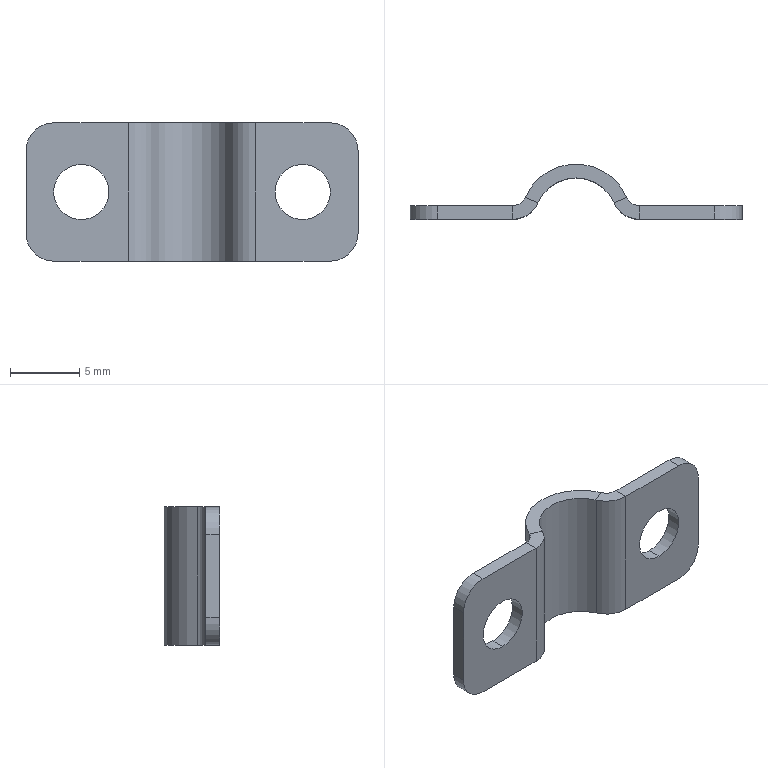Part | NX | features BREP 1 | 1 solid | 30 faces | box 24 x 4 x 10 mm | volume 235.71 mm3 | plane 16 | cylinder 14 | commonest cylinder face diameters 4 x10 2 x2 6 x1 8 x1
STEP:
#1=CARTESIAN_POINT('',(-10.,0.,5.));
#2=VERTEX_POINT('',#1);
#3=CARTESIAN_POINT('',(-12.,0.,3.));
#4=VERTEX_POINT('',#3);
#5=CARTESIAN_POINT('',(-10.,0.,3.));
#6=DIRECTION('',(0.,-1.,0.));
#7=DIRECTION('',(-1.,0.,0.));
#8=AXIS2_PLACEMENT_3D('',#5,#6,#7);
#9=CIRCLE('',#8,2.);
#10=EDGE_CURVE('',#2,#4,#9,.T.);
#11=ORIENTED_EDGE('',*,*,#10,.F.);
#12=CARTESIAN_POINT('',(-10.,1.,5.));
#13=VERTEX_POINT('',#12);
#14=CARTESIAN_POINT('',(-10.,1.6,5.));
#15=DIRECTION('',(0.,-1.,0.));
#16=VECTOR('',#15,1000.);
#17=LINE('',#14,#16);
#18=EDGE_CURVE('',#13,#2,#17,.T.);
#19=ORIENTED_EDGE('',*,*,#18,.F.);
#20=CARTESIAN_POINT('',(-12.,1.,3.));
#21=VERTEX_POINT('',#20);
#22=CARTESIAN_POINT('',(-10.,1.,3.));
#23=DIRECTION('',(0.,1.,0.));
#24=DIRECTION('',(-1.,0.,0.));
#25=AXIS2_PLACEMENT_3D('',#22,#23,#24);
#26=CIRCLE('',#25,2.);
#27=EDGE_CURVE('',#21,#13,#26,.T.);
#28=ORIENTED_EDGE('',*,*,#27,.F.);
#29=CARTESIAN_POINT('',(-12.,0.,3.));
#30=DIRECTION('',(0.,1.,0.));
#31=VECTOR('',#30,1000.);
#32=LINE('',#29,#31);
#33=EDGE_CURVE('',#4,#21,#32,.T.);
#34=ORIENTED_EDGE('',*,*,#33,.F.);
#35=EDGE_LOOP('',(#11,#19,#28,#34));
#36=FACE_BOUND('',#35,.T.);
#37=CARTESIAN_POINT('',(-10.,0.,3.));
#38=DIRECTION('',(0.,1.,0.));
#39=DIRECTION('',(0.,0.,1.));
#40=AXIS2_PLACEMENT_3D('',#37,#38,#39);
#41=CYLINDRICAL_SURFACE('',#40,2.);
#42=ADVANCED_FACE('',(#36),#41,.T.);
#43=CARTESIAN_POINT('',(-12.,0.,-3.));
#44=VERTEX_POINT('',#43);
#45=CARTESIAN_POINT('',(-10.,0.,-5.));
#46=VERTEX_POINT('',#45);
#47=CARTESIAN_POINT('',(-10.,0.,-3.));
#48=DIRECTION('',(0.,-1.,0.));
#49=DIRECTION('',(-1.,0.,0.));
#50=AXIS2_PLACEMENT_3D('',#47,#48,#49);
#51=CIRCLE('',#50,2.);
#52=EDGE_CURVE('',#44,#46,#51,.T.);
#53=ORIENTED_EDGE('',*,*,#52,.F.);
#54=CARTESIAN_POINT('',(-12.,1.,-3.));
#55=VERTEX_POINT('',#54);
#56=CARTESIAN_POINT('',(-12.,0.,-3.));
#57=DIRECTION('',(0.,-1.,0.));
#58=VECTOR('',#57,1000.);
#59=LINE('',#56,#58);
#60=EDGE_CURVE('',#55,#44,#59,.T.);
#61=ORIENTED_EDGE('',*,*,#60,.F.);
#62=CARTESIAN_POINT('',(-10.,1.,-5.));
#63=VERTEX_POINT('',#62);
#64=CARTESIAN_POINT('',(-10.,1.,-3.));
#65=DIRECTION('',(0.,1.,0.));
#66=DIRECTION('',(-1.,0.,0.));
#67=AXIS2_PLACEMENT_3D('',#64,#65,#66);
#68=CIRCLE('',#67,2.);
#69=EDGE_CURVE('',#63,#55,#68,.T.);
#70=ORIENTED_EDGE('',*,*,#69,.F.);
#71=CARTESIAN_POINT('',(-10.,1.,-5.));
#72=DIRECTION('',(0.,1.,0.));
#73=VECTOR('',#72,1000.);
#74=LINE('',#71,#73);
#75=EDGE_CURVE('',#46,#63,#74,.T.);
#76=ORIENTED_EDGE('',*,*,#75,.F.);
#77=EDGE_LOOP('',(#53,#61,#70,#76));
#78=FACE_BOUND('',#77,.T.);
#79=CARTESIAN_POINT('',(-10.,2.,-3.));
#80=DIRECTION('',(0.,-1.,0.));
#81=DIRECTION('',(0.,0.,-1.));
#82=AXIS2_PLACEMENT_3D('',#79,#80,#81);
#83=CYLINDRICAL_SURFACE('',#82,2.);
#84=ADVANCED_FACE('',(#78),#83,.T.);
#85=CARTESIAN_POINT('',(12.,1.,-3.));
#86=VERTEX_POINT('',#85);
#87=CARTESIAN_POINT('',(10.,1.,-5.));
#88=VERTEX_POINT('',#87);
#89=CARTESIAN_POINT('',(10.,1.,-3.));
#90=DIRECTION('',(0.,1.,0.));
#91=DIRECTION('',(-1.,0.,0.));
#92=AXIS2_PLACEMENT_3D('',#89,#90,#91);
#93=CIRCLE('',#92,2.);
#94=EDGE_CURVE('',#86,#88,#93,.T.);
#95=ORIENTED_EDGE('',*,*,#94,.F.);
#96=CARTESIAN_POINT('',(12.,0.,-3.));
#97=VERTEX_POINT('',#96);
#98=CARTESIAN_POINT('',(12.,1.,-3.));
#99=DIRECTION('',(0.,1.,0.));
#100=VECTOR('',#99,1000.);
#101=LINE('',#98,#100);
#102=EDGE_CURVE('',#97,#86,#101,.T.);
#103=ORIENTED_EDGE('',*,*,#102,.F.);
#104=CARTESIAN_POINT('',(10.,0.,-5.));
#105=VERTEX_POINT('',#104);
#106=CARTESIAN_POINT('',(10.,0.,-3.));
#107=DIRECTION('',(0.,-1.,0.));
#108=DIRECTION('',(-1.,0.,0.));
#109=AXIS2_PLACEMENT_3D('',#106,#107,#108);
#110=CIRCLE('',#109,2.);
#111=EDGE_CURVE('',#105,#97,#110,.T.);
#112=ORIENTED_EDGE('',*,*,#111,.F.);
#113=CARTESIAN_POINT('',(10.,1.6,-5.));
#114=DIRECTION('',(0.,-1.,0.));
#115=VECTOR('',#114,1000.);
#116=LINE('',#113,#115);
#117=EDGE_CURVE('',#88,#105,#116,.T.);
#118=ORIENTED_EDGE('',*,*,#117,.F.);
#119=EDGE_LOOP('',(#95,#103,#112,#118));
#120=FACE_BOUND('',#119,.T.);
#121=CARTESIAN_POINT('',(10.,1.6,-3.));
#122=DIRECTION('',(0.,-1.,0.));
#123=DIRECTION('',(0.,0.,-1.));
#124=AXIS2_PLACEMENT_3D('',#121,#122,#123);
#125=CYLINDRICAL_SURFACE('',#124,2.);
#126=ADVANCED_FACE('',(#120),#125,.T.);
#127=CARTESIAN_POINT('',(10.,1.,5.));
#128=VERTEX_POINT('',#127);
#129=CARTESIAN_POINT('',(12.,1.,3.));
#130=VERTEX_POINT('',#129);
#131=CARTESIAN_POINT('',(10.,1.,3.));
#132=DIRECTION('',(0.,1.,0.));
#133=DIRECTION('',(-1.,0.,0.));
#134=AXIS2_PLACEMENT_3D('',#131,#132,#133);
#135=CIRCLE('',#134,2.);
#136=EDGE_CURVE('',#128,#130,#135,.T.);
#137=ORIENTED_EDGE('',*,*,#136,.F.);
#138=CARTESIAN_POINT('',(10.,0.,5.));
#139=VERTEX_POINT('',#138);
#140=CARTESIAN_POINT('',(10.,2.,5.));
#141=DIRECTION('',(0.,1.,0.));
#142=VECTOR('',#141,1000.);
#143=LINE('',#140,#142);
#144=EDGE_CURVE('',#139,#128,#143,.T.);
#145=ORIENTED_EDGE('',*,*,#144,.F.);
#146=CARTESIAN_POINT('',(12.,0.,3.));
#147=VERTEX_POINT('',#146);
#148=CARTESIAN_POINT('',(10.,0.,3.));
#149=DIRECTION('',(0.,-1.,0.));
#150=DIRECTION('',(-1.,0.,0.));
#151=AXIS2_PLACEMENT_3D('',#148,#149,#150);
#152=CIRCLE('',#151,2.);
#153=EDGE_CURVE('',#147,#139,#152,.T.);
#154=ORIENTED_EDGE('',*,*,#153,.F.);
#155=CARTESIAN_POINT('',(12.,1.,3.));
#156=DIRECTION('',(0.,-1.,0.));
#157=VECTOR('',#156,1000.);
#158=LINE('',#155,#157);
#159=EDGE_CURVE('',#130,#147,#158,.T.);
#160=ORIENTED_EDGE('',*,*,#159,.F.);
#161=EDGE_LOOP('',(#137,#145,#154,#160));
#162=FACE_BOUND('',#161,.T.);
#163=CARTESIAN_POINT('',(10.,1.,3.));
#164=DIRECTION('',(0.,-1.,0.));
#165=DIRECTION('',(0.,0.,-1.));
#166=AXIS2_PLACEMENT_3D('',#163,#164,#165);
#167=CYLINDRICAL_SURFACE('',#166,2.);
#168=ADVANCED_FACE('',(#162),#167,.T.);
#169=CARTESIAN_POINT('',(8.,1.,-2.));
#170=VERTEX_POINT('',#169);
#171=CARTESIAN_POINT('',(8.,0.,-2.));
#172=VERTEX_POINT('',#171);
#173=CARTESIAN_POINT('',(8.,1.,-2.));
#174=DIRECTION('',(0.,1.,0.));
#175=VECTOR('',#174,1000.);
#176=LINE('',#173,#175);
#177=EDGE_CURVE('',#170,#172,#176,.F.);
#178=ORIENTED_EDGE('',*,*,#177,.T.);
#179=CARTESIAN_POINT('',(8.,0.,2.));
#180=VERTEX_POINT('',#179);
#181=CARTESIAN_POINT('',(8.,0.,0.));
#182=DIRECTION('',(0.,1.,0.));
#183=DIRECTION('',(-1.,0.,0.));
#184=AXIS2_PLACEMENT_3D('',#181,#182,#183);
#185=CIRCLE('',#184,2.);
#186=EDGE_CURVE('',#180,#172,#185,.T.);
#187=ORIENTED_EDGE('',*,*,#186,.F.);
#188=CARTESIAN_POINT('',(8.,1.,2.));
#189=VERTEX_POINT('',#188);
#190=CARTESIAN_POINT('',(8.,1.,2.));
#191=DIRECTION('',(0.,1.,0.));
#192=VECTOR('',#191,1000.);
#193=LINE('',#190,#192);
#194=EDGE_CURVE('',#189,#180,#193,.F.);
#195=ORIENTED_EDGE('',*,*,#194,.F.);
#196=CARTESIAN_POINT('',(8.,1.,0.));
#197=DIRECTION('',(0.,1.,0.));
#198=DIRECTION('',(0.,0.,1.));
#199=AXIS2_PLACEMENT_3D('',#196,#197,#198);
#200=CIRCLE('',#199,2.);
#201=EDGE_CURVE('',#189,#170,#200,.T.);
#202=ORIENTED_EDGE('',*,*,#201,.T.);
#203=EDGE_LOOP('',(#178,#187,#195,#202));
#204=FACE_BOUND('',#203,.T.);
#205=CARTESIAN_POINT('',(8.,1.,0.));
#206=DIRECTION('',(0.,1.,0.));
#207=DIRECTION('',(0.,0.,1.));
#208=AXIS2_PLACEMENT_3D('',#205,#206,#207);
#209=CYLINDRICAL_SURFACE('',#208,2.);
#210=ADVANCED_FACE('',(#204),#209,.F.);
#211=CARTESIAN_POINT('',(-8.,1.,-2.));
#212=VERTEX_POINT('',#211);
#213=CARTESIAN_POINT('',(-8.,0.,-2.));
#214=VERTEX_POINT('',#213);
#215=CARTESIAN_POINT('',(-8.,1.,-2.));
#216=DIRECTION('',(0.,1.,0.));
#217=VECTOR('',#216,1000.);
#218=LINE('',#215,#217);
#219=EDGE_CURVE('',#212,#214,#218,.F.);
#220=ORIENTED_EDGE('',*,*,#219,.T.);
#221=CARTESIAN_POINT('',(-8.,0.,2.));
#222=VERTEX_POINT('',#221);
#223=CARTESIAN_POINT('',(-8.,0.,0.));
#224=DIRECTION('',(0.,1.,0.));
#225=DIRECTION('',(-1.,0.,0.));
#226=AXIS2_PLACEMENT_3D('',#223,#224,#225);
#227=CIRCLE('',#226,2.);
#228=EDGE_CURVE('',#222,#214,#227,.T.);
#229=ORIENTED_EDGE('',*,*,#228,.F.);
#230=CARTESIAN_POINT('',(-8.,1.,2.));
#231=VERTEX_POINT('',#230);
#232=CARTESIAN_POINT('',(-8.,1.,2.));
#233=DIRECTION('',(0.,1.,0.));
#234=VECTOR('',#233,1000.);
#235=LINE('',#232,#234);
#236=EDGE_CURVE('',#231,#222,#235,.F.);
#237=ORIENTED_EDGE('',*,*,#236,.F.);
#238=CARTESIAN_POINT('',(-8.,1.,0.));
#239=DIRECTION('',(0.,1.,0.));
#240=DIRECTION('',(0.,0.,1.));
#241=AXIS2_PLACEMENT_3D('',#238,#239,#240);
#242=CIRCLE('',#241,2.);
#243=EDGE_CURVE('',#231,#212,#242,.T.);
#244=ORIENTED_EDGE('',*,*,#243,.T.);
#245=EDGE_LOOP('',(#220,#229,#237,#244));
#246=FACE_BOUND('',#245,.T.);
#247=CARTESIAN_POINT('',(-8.,1.,0.));
#248=DIRECTION('',(0.,1.,0.));
#249=DIRECTION('',(0.,0.,1.));
#250=AXIS2_PLACEMENT_3D('',#247,#248,#249);
#251=CYLINDRICAL_SURFACE('',#250,2.);
#252=ADVANCED_FACE('',(#246),#251,.F.);
#253=CARTESIAN_POINT('',(-4.583,0.,-5.));
#254=VERTEX_POINT('',#253);
#255=CARTESIAN_POINT('',(-3.,0.,-5.));
#256=DIRECTION('',(1.,0.,0.));
#257=VECTOR('',#256,1000.);
#258=LINE('',#255,#257);
#259=EDGE_CURVE('',#46,#254,#258,.T.);
#260=ORIENTED_EDGE('',*,*,#259,.F.);
#261=ORIENTED_EDGE('',*,*,#75,.T.);
#262=CARTESIAN_POINT('',(-4.583,1.,-5.));
#263=VERTEX_POINT('',#262);
#264=CARTESIAN_POINT('',(-3.,1.,-5.));
#265=DIRECTION('',(1.,0.,0.));
#266=VECTOR('',#265,1000.);
#267=LINE('',#264,#266);
#268=EDGE_CURVE('',#63,#263,#267,.T.);
#269=ORIENTED_EDGE('',*,*,#268,.T.);
#270=CARTESIAN_POINT('',(-4.583,1.,-5.));
#271=DIRECTION('',(0.,-1.,0.));
#272=VECTOR('',#271,1000.);
#273=LINE('',#270,#272);
#274=EDGE_CURVE('',#263,#254,#273,.T.);
#275=ORIENTED_EDGE('',*,*,#274,.T.);
#276=EDGE_LOOP('',(#260,#261,#269,#275));
#277=FACE_BOUND('',#276,.T.);
#278=CARTESIAN_POINT('',(4.583,2.,-5.));
#279=DIRECTION('',(0.,0.,1.));
#280=DIRECTION('',(1.,0.,0.));
#281=AXIS2_PLACEMENT_3D('',#278,#279,#280);
#282=PLANE('',#281);
#283=ADVANCED_FACE('',(#277),#282,.F.);
#284=CARTESIAN_POINT('',(4.583,0.,5.));
#285=VERTEX_POINT('',#284);
#286=CARTESIAN_POINT('',(3.,0.,5.));
#287=DIRECTION('',(1.,0.,0.));
#288=VECTOR('',#287,1000.);
#289=LINE('',#286,#288);
#290=EDGE_CURVE('',#285,#139,#289,.T.);
#291=ORIENTED_EDGE('',*,*,#290,.T.);
#292=ORIENTED_EDGE('',*,*,#144,.T.);
#293=CARTESIAN_POINT('',(4.583,1.,5.));
#294=VERTEX_POINT('',#293);
#295=CARTESIAN_POINT('',(3.,1.,5.));
#296=DIRECTION('',(1.,0.,0.));
#297=VECTOR('',#296,1000.);
#298=LINE('',#295,#297);
#299=EDGE_CURVE('',#294,#128,#298,.T.);
#300=ORIENTED_EDGE('',*,*,#299,.F.);
#301=CARTESIAN_POINT('',(4.583,1.,5.));
#302=DIRECTION('',(0.,-1.,0.));
#303=VECTOR('',#302,1000.);
#304=LINE('',#301,#303);
#305=EDGE_CURVE('',#294,#285,#304,.T.);
#306=ORIENTED_EDGE('',*,*,#305,.T.);
#307=EDGE_LOOP('',(#291,#292,#300,#306));
#308=FACE_BOUND('',#307,.T.);
#309=CARTESIAN_POINT('',(4.583,2.,5.));
#310=DIRECTION('',(0.,0.,1.));
#311=DIRECTION('',(1.,0.,0.));
#312=AXIS2_PLACEMENT_3D('',#309,#310,#311);
#313=PLANE('',#312);
#314=ADVANCED_FACE('',(#308),#313,.T.);
#315=CARTESIAN_POINT('',(2.75,1.2,-5.));
#316=VERTEX_POINT('',#315);
#317=CARTESIAN_POINT('',(4.583,0.,-5.));
#318=VERTEX_POINT('',#317);
#319=CARTESIAN_POINT('',(4.583,2.,-5.));
#320=DIRECTION('',(0.,0.,1.));
#321=DIRECTION('',(-1.,0.,0.));
#322=AXIS2_PLACEMENT_3D('',#319,#320,#321);
#323=CIRCLE('',#322,2.);
#324=EDGE_CURVE('',#316,#318,#323,.T.);
#325=ORIENTED_EDGE('',*,*,#324,.T.);
#326=CARTESIAN_POINT('',(4.583,0.,5.));
#327=DIRECTION('',(0.,0.,-1.));
#328=VECTOR('',#327,1000.);
#329=LINE('',#326,#328);
#330=EDGE_CURVE('',#285,#318,#329,.T.);
#331=ORIENTED_EDGE('',*,*,#330,.F.);
#332=CARTESIAN_POINT('',(2.75,1.2,5.));
#333=VERTEX_POINT('',#332);
#334=CARTESIAN_POINT('',(4.583,2.,5.));
#335=DIRECTION('',(0.,0.,1.));
#336=DIRECTION('',(-1.,0.,0.));
#337=AXIS2_PLACEMENT_3D('',#334,#335,#336);
#338=CIRCLE('',#337,2.);
#339=EDGE_CURVE('',#333,#285,#338,.T.);
#340=ORIENTED_EDGE('',*,*,#339,.F.);
#341=CARTESIAN_POINT('',(2.75,1.2,5.));
#342=DIRECTION('',(0.,0.,-1.));
#343=VECTOR('',#342,1000.);
#344=LINE('',#341,#343);
#345=EDGE_CURVE('',#333,#316,#344,.T.);
#346=ORIENTED_EDGE('',*,*,#345,.T.);
#347=EDGE_LOOP('',(#325,#331,#340,#346));
#348=FACE_BOUND('',#347,.T.);
#349=CARTESIAN_POINT('',(4.583,2.,5.));
#350=DIRECTION('',(0.,0.,-1.));
#351=DIRECTION('',(-1.,0.,0.));
#352=AXIS2_PLACEMENT_3D('',#349,#350,#351);
#353=CYLINDRICAL_SURFACE('',#352,2.);
#354=ADVANCED_FACE('',(#348),#353,.T.);
#355=CARTESIAN_POINT('',(-2.75,1.2,-5.));
#356=VERTEX_POINT('',#355);
#357=CARTESIAN_POINT('',(0.,0.,-5.));
#358=DIRECTION('',(0.,0.,-1.));
#359=DIRECTION('',(1.,0.,0.));
#360=AXIS2_PLACEMENT_3D('',#357,#358,#359);
#361=CIRCLE('',#360,3.);
#362=EDGE_CURVE('',#356,#316,#361,.T.);
#363=ORIENTED_EDGE('',*,*,#362,.T.);
#364=ORIENTED_EDGE('',*,*,#345,.F.);
#365=CARTESIAN_POINT('',(-2.75,1.2,5.));
#366=VERTEX_POINT('',#365);
#367=CARTESIAN_POINT('',(0.,0.,5.));
#368=DIRECTION('',(0.,0.,-1.));
#369=DIRECTION('',(1.,0.,0.));
#370=AXIS2_PLACEMENT_3D('',#367,#368,#369);
#371=CIRCLE('',#370,3.);
#372=EDGE_CURVE('',#366,#333,#371,.T.);
#373=ORIENTED_EDGE('',*,*,#372,.F.);
#374=CARTESIAN_POINT('',(-2.75,1.2,5.));
#375=DIRECTION('',(0.,0.,-1.));
#376=VECTOR('',#375,1000.);
#377=LINE('',#374,#376);
#378=EDGE_CURVE('',#366,#356,#377,.T.);
#379=ORIENTED_EDGE('',*,*,#378,.T.);
#380=EDGE_LOOP('',(#363,#364,#373,#379));
#381=FACE_BOUND('',#380,.T.);
#382=CARTESIAN_POINT('',(0.,0.,5.));
#383=DIRECTION('',(0.,0.,-1.));
#384=DIRECTION('',(-1.,0.,0.));
#385=AXIS2_PLACEMENT_3D('',#382,#383,#384);
#386=CYLINDRICAL_SURFACE('',#385,3.);
#387=ADVANCED_FACE('',(#381),#386,.F.);
#388=CARTESIAN_POINT('',(-4.583,2.,-5.));
#389=DIRECTION('',(0.,0.,1.));
#390=DIRECTION('',(-1.,0.,0.));
#391=AXIS2_PLACEMENT_3D('',#388,#389,#390);
#392=CIRCLE('',#391,2.);
#393=EDGE_CURVE('',#254,#356,#392,.T.);
#394=ORIENTED_EDGE('',*,*,#393,.T.);
#395=ORIENTED_EDGE('',*,*,#378,.F.);
#396=CARTESIAN_POINT('',(-4.583,0.,5.));
#397=VERTEX_POINT('',#396);
#398=CARTESIAN_POINT('',(-4.583,2.,5.));
#399=DIRECTION('',(0.,0.,1.));
#400=DIRECTION('',(-1.,0.,0.));
#401=AXIS2_PLACEMENT_3D('',#398,#399,#400);
#402=CIRCLE('',#401,2.);
#403=EDGE_CURVE('',#397,#366,#402,.T.);
#404=ORIENTED_EDGE('',*,*,#403,.F.);
#405=CARTESIAN_POINT('',(-4.583,0.,5.));
#406=DIRECTION('',(0.,0.,-1.));
#407=VECTOR('',#406,1000.);
#408=LINE('',#405,#407);
#409=EDGE_CURVE('',#397,#254,#408,.T.);
#410=ORIENTED_EDGE('',*,*,#409,.T.);
#411=EDGE_LOOP('',(#394,#395,#404,#410));
#412=FACE_BOUND('',#411,.T.);
#413=CARTESIAN_POINT('',(-4.583,2.,5.));
#414=DIRECTION('',(0.,0.,-1.));
#415=DIRECTION('',(-1.,0.,0.));
#416=AXIS2_PLACEMENT_3D('',#413,#414,#415);
#417=CYLINDRICAL_SURFACE('',#416,2.);
#418=ADVANCED_FACE('',(#412),#417,.T.);
#419=CARTESIAN_POINT('',(-12.,0.,5.));
#420=DIRECTION('',(0.,0.,-1.));
#421=VECTOR('',#420,1000.);
#422=LINE('',#419,#421);
#423=EDGE_CURVE('',#4,#44,#422,.T.);
#424=ORIENTED_EDGE('',*,*,#423,.T.);
#425=ORIENTED_EDGE('',*,*,#52,.T.);
#426=ORIENTED_EDGE('',*,*,#259,.T.);
#427=ORIENTED_EDGE('',*,*,#409,.F.);
#428=CARTESIAN_POINT('',(-3.,0.,5.));
#429=DIRECTION('',(1.,0.,0.));
#430=VECTOR('',#429,1000.);
#431=LINE('',#428,#430);
#432=EDGE_CURVE('',#2,#397,#431,.T.);
#433=ORIENTED_EDGE('',*,*,#432,.F.);
#434=ORIENTED_EDGE('',*,*,#10,.T.);
#435=EDGE_LOOP('',(#424,#425,#426,#427,#433,#434));
#436=FACE_BOUND('',#435,.T.);
#437=ORIENTED_EDGE('',*,*,#228,.T.);
#438=CARTESIAN_POINT('',(-8.,0.,0.));
#439=DIRECTION('',(0.,1.,0.));
#440=DIRECTION('',(-1.,0.,0.));
#441=AXIS2_PLACEMENT_3D('',#438,#439,#440);
#442=CIRCLE('',#441,2.);
#443=EDGE_CURVE('',#214,#222,#442,.T.);
#444=ORIENTED_EDGE('',*,*,#443,.T.);
#445=EDGE_LOOP('',(#437,#444));
#446=FACE_BOUND('',#445,.T.);
#447=CARTESIAN_POINT('',(-3.,0.,5.));
#448=DIRECTION('',(0.,1.,0.));
#449=DIRECTION('',(-1.,0.,0.));
#450=AXIS2_PLACEMENT_3D('',#447,#448,#449);
#451=PLANE('',#450);
#452=ADVANCED_FACE('',(#436,#446),#451,.F.);
#453=CARTESIAN_POINT('',(-12.,1.,5.));
#454=DIRECTION('',(0.,0.,-1.));
#455=VECTOR('',#454,1000.);
#456=LINE('',#453,#455);
#457=EDGE_CURVE('',#21,#55,#456,.T.);
#458=ORIENTED_EDGE('',*,*,#457,.T.);
#459=ORIENTED_EDGE('',*,*,#60,.T.);
#460=ORIENTED_EDGE('',*,*,#423,.F.);
#461=ORIENTED_EDGE('',*,*,#33,.T.);
#462=EDGE_LOOP('',(#458,#459,#460,#461));
#463=FACE_BOUND('',#462,.T.);
#464=CARTESIAN_POINT('',(-12.,0.,5.));
#465=DIRECTION('',(-1.,0.,0.));
#466=DIRECTION('',(0.,0.,1.));
#467=AXIS2_PLACEMENT_3D('',#464,#465,#466);
#468=PLANE('',#467);
#469=ADVANCED_FACE('',(#463),#468,.T.);
#470=ORIENTED_EDGE('',*,*,#268,.F.);
#471=ORIENTED_EDGE('',*,*,#69,.T.);
#472=ORIENTED_EDGE('',*,*,#457,.F.);
#473=ORIENTED_EDGE('',*,*,#27,.T.);
#474=CARTESIAN_POINT('',(-4.583,1.,5.));
#475=VERTEX_POINT('',#474);
#476=CARTESIAN_POINT('',(-3.,1.,5.));
#477=DIRECTION('',(1.,0.,0.));
#478=VECTOR('',#477,1000.);
#479=LINE('',#476,#478);
#480=EDGE_CURVE('',#13,#475,#479,.T.);
#481=ORIENTED_EDGE('',*,*,#480,.T.);
#482=CARTESIAN_POINT('',(-4.583,1.,5.));
#483=DIRECTION('',(0.,0.,-1.));
#484=VECTOR('',#483,1000.);
#485=LINE('',#482,#484);
#486=EDGE_CURVE('',#475,#263,#485,.T.);
#487=ORIENTED_EDGE('',*,*,#486,.T.);
#488=EDGE_LOOP('',(#470,#471,#472,#473,#481,#487));
#489=FACE_BOUND('',#488,.T.);
#490=ORIENTED_EDGE('',*,*,#243,.F.);
#491=CARTESIAN_POINT('',(-8.,1.,0.));
#492=DIRECTION('',(0.,1.,0.));
#493=DIRECTION('',(0.,0.,1.));
#494=AXIS2_PLACEMENT_3D('',#491,#492,#493);
#495=CIRCLE('',#494,2.);
#496=EDGE_CURVE('',#212,#231,#495,.T.);
#497=ORIENTED_EDGE('',*,*,#496,.F.);
#498=EDGE_LOOP('',(#490,#497));
#499=FACE_BOUND('',#498,.T.);
#500=CARTESIAN_POINT('',(-3.,1.,5.));
#501=DIRECTION('',(0.,1.,0.));
#502=DIRECTION('',(-1.,0.,0.));
#503=AXIS2_PLACEMENT_3D('',#500,#501,#502);
#504=PLANE('',#503);
#505=ADVANCED_FACE('',(#489,#499),#504,.T.);
#506=CARTESIAN_POINT('',(-3.666,1.6,-5.));
#507=VERTEX_POINT('',#506);
#508=CARTESIAN_POINT('',(-4.583,2.,-5.));
#509=DIRECTION('',(0.,0.,1.));
#510=DIRECTION('',(1.,0.,0.));
#511=AXIS2_PLACEMENT_3D('',#508,#509,#510);
#512=CIRCLE('',#511,1.);
#513=EDGE_CURVE('',#263,#507,#512,.T.);
#514=ORIENTED_EDGE('',*,*,#513,.F.);
#515=ORIENTED_EDGE('',*,*,#486,.F.);
#516=CARTESIAN_POINT('',(-3.666,1.6,5.));
#517=VERTEX_POINT('',#516);
#518=CARTESIAN_POINT('',(-4.583,2.,5.));
#519=DIRECTION('',(0.,0.,1.));
#520=DIRECTION('',(1.,0.,0.));
#521=AXIS2_PLACEMENT_3D('',#518,#519,#520);
#522=CIRCLE('',#521,1.);
#523=EDGE_CURVE('',#475,#517,#522,.T.);
#524=ORIENTED_EDGE('',*,*,#523,.T.);
#525=CARTESIAN_POINT('',(-3.666,1.6,5.));
#526=DIRECTION('',(0.,0.,-1.));
#527=VECTOR('',#526,1000.);
#528=LINE('',#525,#527);
#529=EDGE_CURVE('',#517,#507,#528,.T.);
#530=ORIENTED_EDGE('',*,*,#529,.T.);
#531=EDGE_LOOP('',(#514,#515,#524,#530));
#532=FACE_BOUND('',#531,.T.);
#533=CARTESIAN_POINT('',(-4.583,2.,5.));
#534=DIRECTION('',(0.,0.,-1.));
#535=DIRECTION('',(-1.,0.,0.));
#536=AXIS2_PLACEMENT_3D('',#533,#534,#535);
#537=CYLINDRICAL_SURFACE('',#536,1.);
#538=ADVANCED_FACE('',(#532),#537,.F.);
#539=CARTESIAN_POINT('',(3.666,1.6,-5.));
#540=VERTEX_POINT('',#539);
#541=CARTESIAN_POINT('',(0.,0.,-5.));
#542=DIRECTION('',(0.,0.,-1.));
#543=DIRECTION('',(1.,0.,0.));
#544=AXIS2_PLACEMENT_3D('',#541,#542,#543);
#545=CIRCLE('',#544,4.);
#546=EDGE_CURVE('',#507,#540,#545,.T.);
#547=ORIENTED_EDGE('',*,*,#546,.F.);
#548=ORIENTED_EDGE('',*,*,#529,.F.);
#549=CARTESIAN_POINT('',(3.666,1.6,5.));
#550=VERTEX_POINT('',#549);
#551=CARTESIAN_POINT('',(0.,0.,5.));
#552=DIRECTION('',(0.,0.,-1.));
#553=DIRECTION('',(1.,0.,0.));
#554=AXIS2_PLACEMENT_3D('',#551,#552,#553);
#555=CIRCLE('',#554,4.);
#556=EDGE_CURVE('',#517,#550,#555,.T.);
#557=ORIENTED_EDGE('',*,*,#556,.T.);
#558=CARTESIAN_POINT('',(3.666,1.6,5.));
#559=DIRECTION('',(0.,0.,-1.));
#560=VECTOR('',#559,1000.);
#561=LINE('',#558,#560);
#562=EDGE_CURVE('',#550,#540,#561,.T.);
#563=ORIENTED_EDGE('',*,*,#562,.T.);
#564=EDGE_LOOP('',(#547,#548,#557,#563));
#565=FACE_BOUND('',#564,.T.);
#566=CARTESIAN_POINT('',(0.,0.,5.));
#567=DIRECTION('',(0.,0.,-1.));
#568=DIRECTION('',(-1.,0.,0.));
#569=AXIS2_PLACEMENT_3D('',#566,#567,#568);
#570=CYLINDRICAL_SURFACE('',#569,4.);
#571=ADVANCED_FACE('',(#565),#570,.T.);
#572=CARTESIAN_POINT('',(4.583,1.,-5.));
#573=VERTEX_POINT('',#572);
#574=CARTESIAN_POINT('',(4.583,2.,-5.));
#575=DIRECTION('',(0.,0.,1.));
#576=DIRECTION('',(1.,0.,0.));
#577=AXIS2_PLACEMENT_3D('',#574,#575,#576);
#578=CIRCLE('',#577,1.);
#579=EDGE_CURVE('',#540,#573,#578,.T.);
#580=ORIENTED_EDGE('',*,*,#579,.F.);
#581=ORIENTED_EDGE('',*,*,#562,.F.);
#582=CARTESIAN_POINT('',(4.583,2.,5.));
#583=DIRECTION('',(0.,0.,1.));
#584=DIRECTION('',(1.,0.,0.));
#585=AXIS2_PLACEMENT_3D('',#582,#583,#584);
#586=CIRCLE('',#585,1.);
#587=EDGE_CURVE('',#550,#294,#586,.T.);
#588=ORIENTED_EDGE('',*,*,#587,.T.);
#589=CARTESIAN_POINT('',(4.583,1.,5.));
#590=DIRECTION('',(0.,0.,-1.));
#591=VECTOR('',#590,1000.);
#592=LINE('',#589,#591);
#593=EDGE_CURVE('',#294,#573,#592,.T.);
#594=ORIENTED_EDGE('',*,*,#593,.T.);
#595=EDGE_LOOP('',(#580,#581,#588,#594));
#596=FACE_BOUND('',#595,.T.);
#597=CARTESIAN_POINT('',(4.583,2.,5.));
#598=DIRECTION('',(0.,0.,-1.));
#599=DIRECTION('',(-1.,0.,0.));
#600=AXIS2_PLACEMENT_3D('',#597,#598,#599);
#601=CYLINDRICAL_SURFACE('',#600,1.);
#602=ADVANCED_FACE('',(#596),#601,.F.);
#603=ORIENTED_EDGE('',*,*,#299,.T.);
#604=ORIENTED_EDGE('',*,*,#136,.T.);
#605=CARTESIAN_POINT('',(12.,1.,5.));
#606=DIRECTION('',(0.,0.,-1.));
#607=VECTOR('',#606,1000.);
#608=LINE('',#605,#607);
#609=EDGE_CURVE('',#130,#86,#608,.T.);
#610=ORIENTED_EDGE('',*,*,#609,.T.);
#611=ORIENTED_EDGE('',*,*,#94,.T.);
#612=CARTESIAN_POINT('',(3.,1.,-5.));
#613=DIRECTION('',(1.,0.,0.));
#614=VECTOR('',#613,1000.);
#615=LINE('',#612,#614);
#616=EDGE_CURVE('',#573,#88,#615,.T.);
#617=ORIENTED_EDGE('',*,*,#616,.F.);
#618=ORIENTED_EDGE('',*,*,#593,.F.);
#619=EDGE_LOOP('',(#603,#604,#610,#611,#617,#618));
#620=FACE_BOUND('',#619,.T.);
#621=ORIENTED_EDGE('',*,*,#201,.F.);
#622=CARTESIAN_POINT('',(8.,1.,0.));
#623=DIRECTION('',(0.,1.,0.));
#624=DIRECTION('',(0.,0.,1.));
#625=AXIS2_PLACEMENT_3D('',#622,#623,#624);
#626=CIRCLE('',#625,2.);
#627=EDGE_CURVE('',#170,#189,#626,.T.);
#628=ORIENTED_EDGE('',*,*,#627,.F.);
#629=EDGE_LOOP('',(#621,#628));
#630=FACE_BOUND('',#629,.T.);
#631=CARTESIAN_POINT('',(3.,1.,5.));
#632=DIRECTION('',(0.,1.,0.));
#633=DIRECTION('',(-1.,0.,0.));
#634=AXIS2_PLACEMENT_3D('',#631,#632,#633);
#635=PLANE('',#634);
#636=ADVANCED_FACE('',(#620,#630),#635,.T.);
#637=ORIENTED_EDGE('',*,*,#609,.F.);
#638=ORIENTED_EDGE('',*,*,#159,.T.);
#639=CARTESIAN_POINT('',(12.,0.,5.));
#640=DIRECTION('',(0.,0.,-1.));
#641=VECTOR('',#640,1000.);
#642=LINE('',#639,#641);
#643=EDGE_CURVE('',#147,#97,#642,.T.);
#644=ORIENTED_EDGE('',*,*,#643,.T.);
#645=ORIENTED_EDGE('',*,*,#102,.T.);
#646=EDGE_LOOP('',(#637,#638,#644,#645));
#647=FACE_BOUND('',#646,.T.);
#648=CARTESIAN_POINT('',(12.,1.,5.));
#649=DIRECTION('',(1.,0.,0.));
#650=DIRECTION('',(0.,0.,-1.));
#651=AXIS2_PLACEMENT_3D('',#648,#649,#650);
#652=PLANE('',#651);
#653=ADVANCED_FACE('',(#647),#652,.T.);
#654=ORIENTED_EDGE('',*,*,#643,.F.);
#655=ORIENTED_EDGE('',*,*,#153,.T.);
#656=ORIENTED_EDGE('',*,*,#290,.F.);
#657=ORIENTED_EDGE('',*,*,#330,.T.);
#658=CARTESIAN_POINT('',(3.,0.,-5.));
#659=DIRECTION('',(1.,0.,0.));
#660=VECTOR('',#659,1000.);
#661=LINE('',#658,#660);
#662=EDGE_CURVE('',#318,#105,#661,.T.);
#663=ORIENTED_EDGE('',*,*,#662,.T.);
#664=ORIENTED_EDGE('',*,*,#111,.T.);
#665=EDGE_LOOP('',(#654,#655,#656,#657,#663,#664));
#666=FACE_BOUND('',#665,.T.);
#667=ORIENTED_EDGE('',*,*,#186,.T.);
#668=CARTESIAN_POINT('',(8.,0.,0.));
#669=DIRECTION('',(0.,1.,0.));
#670=DIRECTION('',(-1.,0.,0.));
#671=AXIS2_PLACEMENT_3D('',#668,#669,#670);
#672=CIRCLE('',#671,2.);
#673=EDGE_CURVE('',#172,#180,#672,.T.);
#674=ORIENTED_EDGE('',*,*,#673,.T.);
#675=EDGE_LOOP('',(#667,#674));
#676=FACE_BOUND('',#675,.T.);
#677=CARTESIAN_POINT('',(3.,0.,5.));
#678=DIRECTION('',(0.,1.,0.));
#679=DIRECTION('',(-1.,0.,0.));
#680=AXIS2_PLACEMENT_3D('',#677,#678,#679);
#681=PLANE('',#680);
#682=ADVANCED_FACE('',(#666,#676),#681,.F.);
#683=ORIENTED_EDGE('',*,*,#616,.T.);
#684=ORIENTED_EDGE('',*,*,#117,.T.);
#685=ORIENTED_EDGE('',*,*,#662,.F.);
#686=CARTESIAN_POINT('',(4.583,0.,-5.));
#687=DIRECTION('',(0.,1.,0.));
#688=VECTOR('',#687,1000.);
#689=LINE('',#686,#688);
#690=EDGE_CURVE('',#318,#573,#689,.T.);
#691=ORIENTED_EDGE('',*,*,#690,.T.);
#692=EDGE_LOOP('',(#683,#684,#685,#691));
#693=FACE_BOUND('',#692,.T.);
#694=CARTESIAN_POINT('',(3.666,1.6,-5.));
#695=DIRECTION('',(0.,0.,-1.));
#696=DIRECTION('',(-1.,0.,0.));
#697=AXIS2_PLACEMENT_3D('',#694,#695,#696);
#698=PLANE('',#697);
#699=ADVANCED_FACE('',(#693),#698,.T.);
#700=ORIENTED_EDGE('',*,*,#690,.F.);
#701=ORIENTED_EDGE('',*,*,#324,.F.);
#702=CARTESIAN_POINT('',(3.666,1.6,-5.));
#703=DIRECTION('',(-0.9165,-0.4,0.));
#704=VECTOR('',#703,1000.);
#705=LINE('',#702,#704);
#706=EDGE_CURVE('',#540,#316,#705,.T.);
#707=ORIENTED_EDGE('',*,*,#706,.F.);
#708=ORIENTED_EDGE('',*,*,#579,.T.);
#709=EDGE_LOOP('',(#700,#701,#707,#708));
#710=FACE_BOUND('',#709,.T.);
#711=CARTESIAN_POINT('',(4.583,0.,-5.));
#712=DIRECTION('',(0.,0.,-1.));
#713=DIRECTION('',(-1.,0.,0.));
#714=AXIS2_PLACEMENT_3D('',#711,#712,#713);
#715=PLANE('',#714);
#716=ADVANCED_FACE('',(#710),#715,.T.);
#717=ORIENTED_EDGE('',*,*,#372,.T.);
#718=CARTESIAN_POINT('',(2.75,1.2,5.));
#719=DIRECTION('',(0.9165,0.4,0.));
#720=VECTOR('',#719,1000.);
#721=LINE('',#718,#720);
#722=EDGE_CURVE('',#333,#550,#721,.T.);
#723=ORIENTED_EDGE('',*,*,#722,.T.);
#724=ORIENTED_EDGE('',*,*,#556,.F.);
#725=CARTESIAN_POINT('',(-3.666,1.6,5.));
#726=DIRECTION('',(0.9165,-0.4,0.));
#727=VECTOR('',#726,1000.);
#728=LINE('',#725,#727);
#729=EDGE_CURVE('',#517,#366,#728,.T.);
#730=ORIENTED_EDGE('',*,*,#729,.T.);
#731=EDGE_LOOP('',(#717,#723,#724,#730));
#732=FACE_BOUND('',#731,.T.);
#733=CARTESIAN_POINT('',(4.583,1.,5.));
#734=DIRECTION('',(0.,0.,1.));
#735=DIRECTION('',(1.,0.,0.));
#736=AXIS2_PLACEMENT_3D('',#733,#734,#735);
#737=PLANE('',#736);
#738=ADVANCED_FACE('',(#732),#737,.T.);
#739=ORIENTED_EDGE('',*,*,#722,.F.);
#740=ORIENTED_EDGE('',*,*,#339,.T.);
#741=ORIENTED_EDGE('',*,*,#305,.F.);
#742=ORIENTED_EDGE('',*,*,#587,.F.);
#743=EDGE_LOOP('',(#739,#740,#741,#742));
#744=FACE_BOUND('',#743,.T.);
#745=CARTESIAN_POINT('',(2.75,1.2,5.));
#746=DIRECTION('',(0.,0.,1.));
#747=DIRECTION('',(1.,0.,0.));
#748=AXIS2_PLACEMENT_3D('',#745,#746,#747);
#749=PLANE('',#748);
#750=ADVANCED_FACE('',(#744),#749,.T.);
#751=ORIENTED_EDGE('',*,*,#362,.F.);
#752=CARTESIAN_POINT('',(-2.75,1.2,-5.));
#753=DIRECTION('',(-0.9165,0.4,0.));
#754=VECTOR('',#753,1000.);
#755=LINE('',#752,#754);
#756=EDGE_CURVE('',#356,#507,#755,.T.);
#757=ORIENTED_EDGE('',*,*,#756,.T.);
#758=ORIENTED_EDGE('',*,*,#546,.T.);
#759=ORIENTED_EDGE('',*,*,#706,.T.);
#760=EDGE_LOOP('',(#751,#757,#758,#759));
#761=FACE_BOUND('',#760,.T.);
#762=CARTESIAN_POINT('',(-4.583,1.,-5.));
#763=DIRECTION('',(0.,0.,-1.));
#764=DIRECTION('',(-1.,0.,0.));
#765=AXIS2_PLACEMENT_3D('',#762,#763,#764);
#766=PLANE('',#765);
#767=ADVANCED_FACE('',(#761),#766,.T.);
#768=ORIENTED_EDGE('',*,*,#756,.F.);
#769=ORIENTED_EDGE('',*,*,#393,.F.);
#770=ORIENTED_EDGE('',*,*,#274,.F.);
#771=ORIENTED_EDGE('',*,*,#513,.T.);
#772=EDGE_LOOP('',(#768,#769,#770,#771));
#773=FACE_BOUND('',#772,.T.);
#774=CARTESIAN_POINT('',(-2.75,1.2,-5.));
#775=DIRECTION('',(0.,0.,-1.));
#776=DIRECTION('',(-1.,0.,0.));
#777=AXIS2_PLACEMENT_3D('',#774,#775,#776);
#778=PLANE('',#777);
#779=ADVANCED_FACE('',(#773),#778,.T.);
#780=ORIENTED_EDGE('',*,*,#480,.F.);
#781=ORIENTED_EDGE('',*,*,#18,.T.);
#782=ORIENTED_EDGE('',*,*,#432,.T.);
#783=CARTESIAN_POINT('',(-4.583,0.,5.));
#784=DIRECTION('',(0.,1.,0.));
#785=VECTOR('',#784,1000.);
#786=LINE('',#783,#785);
#787=EDGE_CURVE('',#397,#475,#786,.T.);
#788=ORIENTED_EDGE('',*,*,#787,.T.);
#789=EDGE_LOOP('',(#780,#781,#782,#788));
#790=FACE_BOUND('',#789,.T.);
#791=CARTESIAN_POINT('',(-3.666,1.6,5.));
#792=DIRECTION('',(0.,0.,1.));
#793=DIRECTION('',(1.,0.,0.));
#794=AXIS2_PLACEMENT_3D('',#791,#792,#793);
#795=PLANE('',#794);
#796=ADVANCED_FACE('',(#790),#795,.T.);
#797=ORIENTED_EDGE('',*,*,#787,.F.);
#798=ORIENTED_EDGE('',*,*,#403,.T.);
#799=ORIENTED_EDGE('',*,*,#729,.F.);
#800=ORIENTED_EDGE('',*,*,#523,.F.);
#801=EDGE_LOOP('',(#797,#798,#799,#800));
#802=FACE_BOUND('',#801,.T.);
#803=CARTESIAN_POINT('',(-4.583,0.,5.));
#804=DIRECTION('',(0.,0.,1.));
#805=DIRECTION('',(1.,0.,0.));
#806=AXIS2_PLACEMENT_3D('',#803,#804,#805);
#807=PLANE('',#806);
#808=ADVANCED_FACE('',(#802),#807,.T.);
#809=ORIENTED_EDGE('',*,*,#443,.F.);
#810=ORIENTED_EDGE('',*,*,#219,.F.);
#811=ORIENTED_EDGE('',*,*,#496,.T.);
#812=ORIENTED_EDGE('',*,*,#236,.T.);
#813=EDGE_LOOP('',(#809,#810,#811,#812));
#814=FACE_BOUND('',#813,.T.);
#815=CARTESIAN_POINT('',(-8.,1.,0.));
#816=DIRECTION('',(0.,1.,0.));
#817=DIRECTION('',(0.,0.,1.));
#818=AXIS2_PLACEMENT_3D('',#815,#816,#817);
#819=CYLINDRICAL_SURFACE('',#818,2.);
#820=ADVANCED_FACE('',(#814),#819,.F.);
#821=ORIENTED_EDGE('',*,*,#673,.F.);
#822=ORIENTED_EDGE('',*,*,#177,.F.);
#823=ORIENTED_EDGE('',*,*,#627,.T.);
#824=ORIENTED_EDGE('',*,*,#194,.T.);
#825=EDGE_LOOP('',(#821,#822,#823,#824));
#826=FACE_BOUND('',#825,.T.);
#827=CARTESIAN_POINT('',(8.,1.,0.));
#828=DIRECTION('',(0.,1.,0.));
#829=DIRECTION('',(0.,0.,1.));
#830=AXIS2_PLACEMENT_3D('',#827,#828,#829);
#831=CYLINDRICAL_SURFACE('',#830,2.);
#832=ADVANCED_FACE('',(#826),#831,.F.);
#833=CLOSED_SHELL('',(#42,#84,#126,#168,#210,#252,#283,#314,#354,#387,#418,#452,#469,#505,#538,#571,#602,#636,#653,#682,#699,#716,#738,#750,#767,#779,#796,#808,#820,#832));
#834=MANIFOLD_SOLID_BREP('',#833);
#835=(LENGTH_UNIT()NAMED_UNIT(*)SI_UNIT(.MILLI.,.METRE.));
#836=UNCERTAINTY_MEASURE_WITH_UNIT(LENGTH_MEASURE(0.00001),#835,'','');
#837=(NAMED_UNIT(*)PLANE_ANGLE_UNIT()SI_UNIT($,.RADIAN.));
#838=(NAMED_UNIT(*)SI_UNIT($,.STERADIAN.)SOLID_ANGLE_UNIT());
#839=(GEOMETRIC_REPRESENTATION_CONTEXT(3)GLOBAL_UNCERTAINTY_ASSIGNED_CONTEXT((#836))GLOBAL_UNIT_ASSIGNED_CONTEXT((#835,#837,#838))REPRESENTATION_CONTEXT('',''));
#840=ADVANCED_BREP_SHAPE_REPRESENTATION('',(#834),#839);